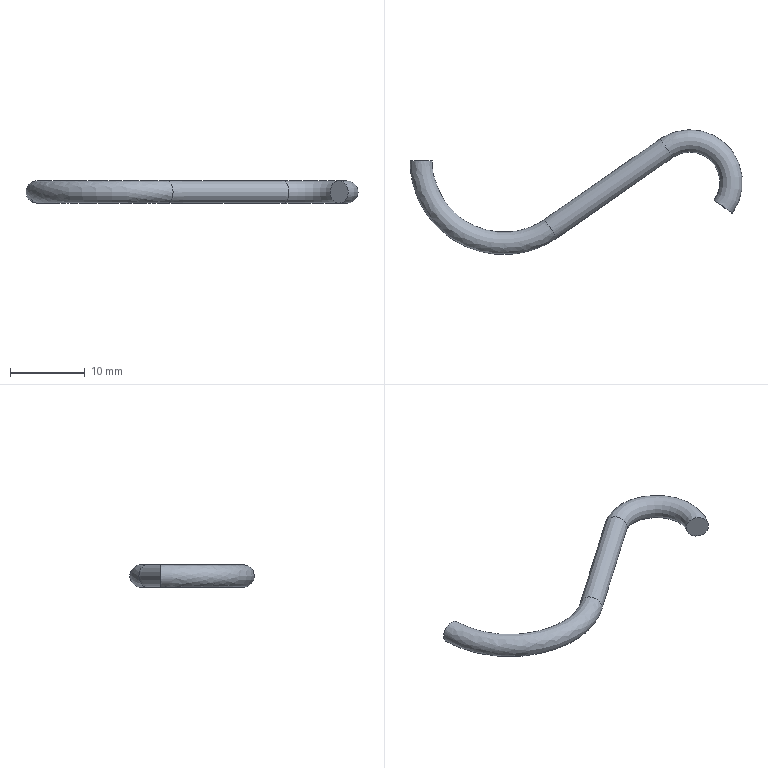Part | NX | features solid 2 | 1 solid | 5 faces | box 44.332 x 16.664 x 3 mm | volume 411.72 mm3 | spline 3 | plane 2
STEP:
#1=CARTESIAN_POINT('',(-1509.519,408.01,-17.5));
#2=VERTEX_POINT('',#1);
#3=CARTESIAN_POINT('',(-1510.727,408.9,-17.5));
#4=DIRECTION('',(-0.5934,-0.8049,0.));
#5=DIRECTION('',(0.8049,-0.5934,0.));
#6=AXIS2_PLACEMENT_3D('',#3,#4,#5);
#7=CIRCLE('',#6,1.5);
#8=EDGE_CURVE('',#2,#2,#7,.T.);
#9=ORIENTED_EDGE('',*,*,#8,.T.);
#10=EDGE_LOOP('',(#9));
#11=FACE_BOUND('',#10,.T.);
#12=CARTESIAN_POINT('',(-1510.727,408.9,-17.5));
#13=DIRECTION('',(0.5934,0.8049,0.));
#14=DIRECTION('',(-0.8049,0.5934,0.));
#15=AXIS2_PLACEMENT_3D('',#12,#13,#14);
#16=PLANE('',#15);
#17=ADVANCED_FACE('',(#11),#16,.F.);
#18=CARTESIAN_POINT('',(-1518.27,416.696,-16.));
#19=VERTEX_POINT('',#18);
#20=CARTESIAN_POINT('',(-1517.968,416.26,-16.));
#21=CARTESIAN_POINT('',(-1518.572,417.131,-16.));
#22=CARTESIAN_POINT('',(-1518.973,417.711,-16.265));
#23=CARTESIAN_POINT('',(-1519.124,417.929,-16.97));
#24=CARTESIAN_POINT('',(-1519.124,417.929,-18.03));
#25=CARTESIAN_POINT('',(-1518.973,417.711,-18.735));
#26=CARTESIAN_POINT('',(-1518.572,417.131,-19.));
#27=CARTESIAN_POINT('',(-1517.968,416.26,-19.));
#28=CARTESIAN_POINT('',(-1517.567,415.68,-18.735));
#29=CARTESIAN_POINT('',(-1517.416,415.462,-18.03));
#30=CARTESIAN_POINT('',(-1517.416,415.462,-16.97));
#31=CARTESIAN_POINT('',(-1517.567,415.68,-16.265));
#32=CARTESIAN_POINT('',(-1517.968,416.26,-16.));
#33=CARTESIAN_POINT('',(-1518.572,417.131,-16.));
#34=(BOUNDED_CURVE()B_SPLINE_CURVE(4,(#20,#21,#22,#23,#24,#25,#26,#27,#28,#29,#30,#31,#32,#33),.UNSPECIFIED.,.T.,.F.)B_SPLINE_CURVE_WITH_KNOTS((2,3,3,3,3,3,2),(-0.25,0.,0.25,0.5,0.75,1.,1.25),.UNSPECIFIED.)CURVE()GEOMETRIC_REPRESENTATION_ITEM()RATIONAL_B_SPLINE_CURVE((1.017,1.017,0.9585,1.017,1.017,0.9585,1.017,1.017,0.9585,1.017,1.017,0.9585,1.017,1.017))REPRESENTATION_ITEM(''));
#35=EDGE_CURVE('',#19,#19,#34,.F.);
#36=ORIENTED_EDGE('',*,*,#35,.T.);
#37=EDGE_LOOP('',(#36));
#38=FACE_BOUND('',#37,.T.);
#39=ORIENTED_EDGE('',*,*,#8,.F.);
#40=EDGE_LOOP('',(#39));
#41=FACE_BOUND('',#40,.T.);
#42=CARTESIAN_POINT('',(-1517.968,416.26,-16.));
#43=CARTESIAN_POINT('',(-1517.914,416.296,-16.));
#44=CARTESIAN_POINT('',(-1517.863,416.33,-16.));
#45=CARTESIAN_POINT('',(-1517.478,416.575,-16.));
#46=CARTESIAN_POINT('',(-1516.983,416.819,-16.));
#47=CARTESIAN_POINT('',(-1515.796,417.144,-16.));
#48=CARTESIAN_POINT('',(-1514.851,417.214,-16.));
#49=CARTESIAN_POINT('',(-1513.213,416.821,-16.));
#50=CARTESIAN_POINT('',(-1512.432,416.392,-16.));
#51=CARTESIAN_POINT('',(-1511.306,415.394,-16.));
#52=CARTESIAN_POINT('',(-1509.795,413.389,-16.));
#53=CARTESIAN_POINT('',(-1510.171,410.387,-16.));
#54=CARTESIAN_POINT('',(-1511.153,409.215,-16.));
#55=CARTESIAN_POINT('',(-1518.572,417.131,-16.));
#56=CARTESIAN_POINT('',(-1518.513,417.171,-16.));
#57=CARTESIAN_POINT('',(-1518.454,417.21,-16.));
#58=CARTESIAN_POINT('',(-1517.931,417.546,-16.));
#59=CARTESIAN_POINT('',(-1517.422,417.778,-16.));
#60=CARTESIAN_POINT('',(-1515.889,418.237,-16.));
#61=CARTESIAN_POINT('',(-1514.813,418.274,-16.));
#62=CARTESIAN_POINT('',(-1512.795,417.818,-16.));
#63=CARTESIAN_POINT('',(-1511.852,417.295,-16.));
#64=CARTESIAN_POINT('',(-1510.485,416.084,-16.));
#65=CARTESIAN_POINT('',(-1508.652,413.65,-16.));
#66=CARTESIAN_POINT('',(-1509.108,410.008,-16.));
#67=CARTESIAN_POINT('',(-1510.3,408.585,-16.));
#68=CARTESIAN_POINT('',(-1518.973,417.711,-16.265));
#69=CARTESIAN_POINT('',(-1518.912,417.752,-16.265));
#70=CARTESIAN_POINT('',(-1518.847,417.795,-16.265));
#71=CARTESIAN_POINT('',(-1518.232,418.191,-16.265));
#72=CARTESIAN_POINT('',(-1517.715,418.416,-16.265));
#73=CARTESIAN_POINT('',(-1515.951,418.963,-16.265));
#74=CARTESIAN_POINT('',(-1514.788,418.977,-16.265));
#75=CARTESIAN_POINT('',(-1512.516,418.481,-16.265));
#76=CARTESIAN_POINT('',(-1511.466,417.894,-16.265));
#77=CARTESIAN_POINT('',(-1509.939,416.542,-16.265));
#78=CARTESIAN_POINT('',(-1507.892,413.824,-16.265));
#79=CARTESIAN_POINT('',(-1508.402,409.757,-16.265));
#80=CARTESIAN_POINT('',(-1509.733,408.167,-16.265));
#81=CARTESIAN_POINT('',(-1519.124,417.929,-16.97));
#82=CARTESIAN_POINT('',(-1519.061,417.971,-16.97));
#83=CARTESIAN_POINT('',(-1518.994,418.016,-16.97));
#84=CARTESIAN_POINT('',(-1518.346,418.434,-16.97));
#85=CARTESIAN_POINT('',(-1517.824,418.655,-16.97));
#86=CARTESIAN_POINT('',(-1515.974,419.237,-16.97));
#87=CARTESIAN_POINT('',(-1514.779,419.242,-16.97));
#88=CARTESIAN_POINT('',(-1512.412,418.73,-16.97));
#89=CARTESIAN_POINT('',(-1511.321,418.12,-16.97));
#90=CARTESIAN_POINT('',(-1509.734,416.714,-16.97));
#91=CARTESIAN_POINT('',(-1507.606,413.89,-16.97));
#92=CARTESIAN_POINT('',(-1508.136,409.662,-16.97));
#93=CARTESIAN_POINT('',(-1509.519,408.01,-16.97));
#94=CARTESIAN_POINT('',(-1519.124,417.929,-18.03));
#95=CARTESIAN_POINT('',(-1519.061,417.971,-18.03));
#96=CARTESIAN_POINT('',(-1518.994,418.016,-18.03));
#97=CARTESIAN_POINT('',(-1518.346,418.434,-18.03));
#98=CARTESIAN_POINT('',(-1517.824,418.655,-18.03));
#99=CARTESIAN_POINT('',(-1515.974,419.237,-18.03));
#100=CARTESIAN_POINT('',(-1514.779,419.242,-18.03));
#101=CARTESIAN_POINT('',(-1512.412,418.73,-18.03));
#102=CARTESIAN_POINT('',(-1511.321,418.12,-18.03));
#103=CARTESIAN_POINT('',(-1509.734,416.714,-18.03));
#104=CARTESIAN_POINT('',(-1507.606,413.89,-18.03));
#105=CARTESIAN_POINT('',(-1508.136,409.662,-18.03));
#106=CARTESIAN_POINT('',(-1509.519,408.01,-18.03));
#107=CARTESIAN_POINT('',(-1518.973,417.711,-18.735));
#108=CARTESIAN_POINT('',(-1518.912,417.752,-18.735));
#109=CARTESIAN_POINT('',(-1518.847,417.795,-18.735));
#110=CARTESIAN_POINT('',(-1518.232,418.191,-18.735));
#111=CARTESIAN_POINT('',(-1517.715,418.416,-18.735));
#112=CARTESIAN_POINT('',(-1515.951,418.963,-18.735));
#113=CARTESIAN_POINT('',(-1514.788,418.977,-18.735));
#114=CARTESIAN_POINT('',(-1512.516,418.481,-18.735));
#115=CARTESIAN_POINT('',(-1511.466,417.894,-18.735));
#116=CARTESIAN_POINT('',(-1509.939,416.542,-18.735));
#117=CARTESIAN_POINT('',(-1507.892,413.824,-18.735));
#118=CARTESIAN_POINT('',(-1508.402,409.757,-18.735));
#119=CARTESIAN_POINT('',(-1509.733,408.167,-18.735));
#120=CARTESIAN_POINT('',(-1518.572,417.131,-19.));
#121=CARTESIAN_POINT('',(-1518.513,417.171,-19.));
#122=CARTESIAN_POINT('',(-1518.454,417.21,-19.));
#123=CARTESIAN_POINT('',(-1517.931,417.546,-19.));
#124=CARTESIAN_POINT('',(-1517.422,417.778,-19.));
#125=CARTESIAN_POINT('',(-1515.889,418.237,-19.));
#126=CARTESIAN_POINT('',(-1514.813,418.274,-19.));
#127=CARTESIAN_POINT('',(-1512.795,417.818,-19.));
#128=CARTESIAN_POINT('',(-1511.852,417.295,-19.));
#129=CARTESIAN_POINT('',(-1510.485,416.084,-19.));
#130=CARTESIAN_POINT('',(-1508.652,413.65,-19.));
#131=CARTESIAN_POINT('',(-1509.108,410.008,-19.));
#132=CARTESIAN_POINT('',(-1510.3,408.585,-19.));
#133=CARTESIAN_POINT('',(-1517.968,416.26,-19.));
#134=CARTESIAN_POINT('',(-1517.914,416.296,-19.));
#135=CARTESIAN_POINT('',(-1517.863,416.33,-19.));
#136=CARTESIAN_POINT('',(-1517.478,416.575,-19.));
#137=CARTESIAN_POINT('',(-1516.983,416.819,-19.));
#138=CARTESIAN_POINT('',(-1515.796,417.144,-19.));
#139=CARTESIAN_POINT('',(-1514.851,417.214,-19.));
#140=CARTESIAN_POINT('',(-1513.213,416.821,-19.));
#141=CARTESIAN_POINT('',(-1512.432,416.392,-19.));
#142=CARTESIAN_POINT('',(-1511.306,415.394,-19.));
#143=CARTESIAN_POINT('',(-1509.795,413.389,-19.));
#144=CARTESIAN_POINT('',(-1510.171,410.387,-19.));
#145=CARTESIAN_POINT('',(-1511.153,409.215,-19.));
#146=CARTESIAN_POINT('',(-1517.567,415.68,-18.735));
#147=CARTESIAN_POINT('',(-1517.516,415.715,-18.735));
#148=CARTESIAN_POINT('',(-1517.471,415.745,-18.735));
#149=CARTESIAN_POINT('',(-1517.176,415.93,-18.735));
#150=CARTESIAN_POINT('',(-1516.691,416.182,-18.735));
#151=CARTESIAN_POINT('',(-1515.734,416.418,-18.735));
#152=CARTESIAN_POINT('',(-1514.875,416.511,-18.735));
#153=CARTESIAN_POINT('',(-1513.492,416.159,-18.735));
#154=CARTESIAN_POINT('',(-1512.818,415.793,-18.735));
#155=CARTESIAN_POINT('',(-1511.851,414.936,-18.735));
#156=CARTESIAN_POINT('',(-1510.555,413.215,-18.735));
#157=CARTESIAN_POINT('',(-1510.878,410.639,-18.735));
#158=CARTESIAN_POINT('',(-1511.721,409.633,-18.735));
#159=CARTESIAN_POINT('',(-1517.416,415.462,-18.03));
#160=CARTESIAN_POINT('',(-1517.366,415.496,-18.03));
#161=CARTESIAN_POINT('',(-1517.323,415.525,-18.03));
#162=CARTESIAN_POINT('',(-1517.063,415.688,-18.03));
#163=CARTESIAN_POINT('',(-1516.581,415.942,-18.03));
#164=CARTESIAN_POINT('',(-1515.71,416.145,-18.03));
#165=CARTESIAN_POINT('',(-1514.885,416.246,-18.03));
#166=CARTESIAN_POINT('',(-1513.596,415.909,-18.03));
#167=CARTESIAN_POINT('',(-1512.963,415.568,-18.03));
#168=CARTESIAN_POINT('',(-1512.057,414.764,-18.03));
#169=CARTESIAN_POINT('',(-1510.841,413.15,-18.03));
#170=CARTESIAN_POINT('',(-1511.144,410.734,-18.03));
#171=CARTESIAN_POINT('',(-1511.934,409.79,-18.03));
#172=CARTESIAN_POINT('',(-1517.416,415.462,-16.97));
#173=CARTESIAN_POINT('',(-1517.366,415.496,-16.97));
#174=CARTESIAN_POINT('',(-1517.323,415.525,-16.97));
#175=CARTESIAN_POINT('',(-1517.063,415.688,-16.97));
#176=CARTESIAN_POINT('',(-1516.581,415.942,-16.97));
#177=CARTESIAN_POINT('',(-1515.71,416.145,-16.97));
#178=CARTESIAN_POINT('',(-1514.885,416.246,-16.97));
#179=CARTESIAN_POINT('',(-1513.596,415.909,-16.97));
#180=CARTESIAN_POINT('',(-1512.963,415.568,-16.97));
#181=CARTESIAN_POINT('',(-1512.057,414.764,-16.97));
#182=CARTESIAN_POINT('',(-1510.841,413.15,-16.97));
#183=CARTESIAN_POINT('',(-1511.144,410.734,-16.97));
#184=CARTESIAN_POINT('',(-1511.934,409.79,-16.97));
#185=CARTESIAN_POINT('',(-1517.567,415.68,-16.265));
#186=CARTESIAN_POINT('',(-1517.516,415.715,-16.265));
#187=CARTESIAN_POINT('',(-1517.471,415.745,-16.265));
#188=CARTESIAN_POINT('',(-1517.176,415.93,-16.265));
#189=CARTESIAN_POINT('',(-1516.691,416.182,-16.265));
#190=CARTESIAN_POINT('',(-1515.734,416.418,-16.265));
#191=CARTESIAN_POINT('',(-1514.875,416.511,-16.265));
#192=CARTESIAN_POINT('',(-1513.492,416.159,-16.265));
#193=CARTESIAN_POINT('',(-1512.818,415.793,-16.265));
#194=CARTESIAN_POINT('',(-1511.851,414.936,-16.265));
#195=CARTESIAN_POINT('',(-1510.555,413.215,-16.265));
#196=CARTESIAN_POINT('',(-1510.878,410.639,-16.265));
#197=CARTESIAN_POINT('',(-1511.721,409.633,-16.265));
#198=CARTESIAN_POINT('',(-1517.968,416.26,-16.));
#199=CARTESIAN_POINT('',(-1517.914,416.296,-16.));
#200=CARTESIAN_POINT('',(-1517.863,416.33,-16.));
#201=CARTESIAN_POINT('',(-1517.478,416.575,-16.));
#202=CARTESIAN_POINT('',(-1516.983,416.819,-16.));
#203=CARTESIAN_POINT('',(-1515.796,417.144,-16.));
#204=CARTESIAN_POINT('',(-1514.851,417.214,-16.));
#205=CARTESIAN_POINT('',(-1513.213,416.821,-16.));
#206=CARTESIAN_POINT('',(-1512.432,416.392,-16.));
#207=CARTESIAN_POINT('',(-1511.306,415.394,-16.));
#208=CARTESIAN_POINT('',(-1509.795,413.389,-16.));
#209=CARTESIAN_POINT('',(-1510.171,410.387,-16.));
#210=CARTESIAN_POINT('',(-1511.153,409.215,-16.));
#211=CARTESIAN_POINT('',(-1518.572,417.131,-16.));
#212=CARTESIAN_POINT('',(-1518.513,417.171,-16.));
#213=CARTESIAN_POINT('',(-1518.454,417.21,-16.));
#214=CARTESIAN_POINT('',(-1517.931,417.546,-16.));
#215=CARTESIAN_POINT('',(-1517.422,417.778,-16.));
#216=CARTESIAN_POINT('',(-1515.889,418.237,-16.));
#217=CARTESIAN_POINT('',(-1514.813,418.274,-16.));
#218=CARTESIAN_POINT('',(-1512.795,417.818,-16.));
#219=CARTESIAN_POINT('',(-1511.852,417.295,-16.));
#220=CARTESIAN_POINT('',(-1510.485,416.084,-16.));
#221=CARTESIAN_POINT('',(-1508.652,413.65,-16.));
#222=CARTESIAN_POINT('',(-1509.108,410.008,-16.));
#223=CARTESIAN_POINT('',(-1510.3,408.585,-16.));
#224=(BOUNDED_SURFACE()B_SPLINE_SURFACE(4,3,((#42,#43,#44,#45,#46,#47,#48,#49,#50,#51,#52,#53,#54),(#55,#56,#57,#58,#59,#60,#61,#62,#63,#64,#65,#66,#67),(#68,#69,#70,#71,#72,#73,#74,#75,#76,#77,#78,#79,#80),(#81,#82,#83,#84,#85,#86,#87,#88,#89,#90,#91,#92,#93),(#94,#95,#96,#97,#98,#99,#100,#101,#102,#103,#104,#105,#106),(#107,#108,#109,#110,#111,#112,#113,#114,#115,#116,#117,#118,#119),(#120,#121,#122,#123,#124,#125,#126,#127,#128,#129,#130,#131,#132),(#133,#134,#135,#136,#137,#138,#139,#140,#141,#142,#143,#144,#145),(#146,#147,#148,#149,#150,#151,#152,#153,#154,#155,#156,#157,#158),(#159,#160,#161,#162,#163,#164,#165,#166,#167,#168,#169,#170,#171),(#172,#173,#174,#175,#176,#177,#178,#179,#180,#181,#182,#183,#184),(#185,#186,#187,#188,#189,#190,#191,#192,#193,#194,#195,#196,#197),(#198,#199,#200,#201,#202,#203,#204,#205,#206,#207,#208,#209,#210),(#211,#212,#213,#214,#215,#216,#217,#218,#219,#220,#221,#222,#223)),.UNSPECIFIED.,.T.,.F.,.F.)B_SPLINE_SURFACE_WITH_KNOTS((2,3,3,3,3,3,2),(4,2,2,2,2,1,4),(-0.25,0.,0.25,0.5,0.75,1.,1.25),(0.,0.01356,0.1166,0.2933,0.47,0.6466,1.),.UNSPECIFIED.)GEOMETRIC_REPRESENTATION_ITEM()RATIONAL_B_SPLINE_SURFACE(((1.017,1.017,1.017,1.017,1.017,1.017,1.017,1.017,1.017,1.017,1.017,1.017,1.017),(1.017,1.017,1.017,1.017,1.017,1.017,1.017,1.017,1.017,1.017,1.017,1.017,1.017),(0.9585,0.9585,0.9585,0.9585,0.9585,0.9585,0.9585,0.9585,0.9585,0.9585,0.9585,0.9585,0.9585),(1.017,1.017,1.017,1.017,1.017,1.017,1.017,1.017,1.017,1.017,1.017,1.017,1.017),(1.017,1.017,1.017,1.017,1.017,1.017,1.017,1.017,1.017,1.017,1.017,1.017,1.017),(0.9585,0.9585,0.9585,0.9585,0.9585,0.9585,0.9585,0.9585,0.9585,0.9585,0.9585,0.9585,0.9585),(1.017,1.017,1.017,1.017,1.017,1.017,1.017,1.017,1.017,1.017,1.017,1.017,1.017),(1.017,1.017,1.017,1.017,1.017,1.017,1.017,1.017,1.017,1.017,1.017,1.017,1.017),(0.9585,0.9585,0.9585,0.9585,0.9585,0.9585,0.9585,0.9585,0.9585,0.9585,0.9585,0.9585,0.9585),(1.017,1.017,1.017,1.017,1.017,1.017,1.017,1.017,1.017,1.017,1.017,1.017,1.017),(1.017,1.017,1.017,1.017,1.017,1.017,1.017,1.017,1.017,1.017,1.017,1.017,1.017),(0.9585,0.9585,0.9585,0.9585,0.9585,0.9585,0.9585,0.9585,0.9585,0.9585,0.9585,0.9585,0.9585),(1.017,1.017,1.017,1.017,1.017,1.017,1.017,1.017,1.017,1.017,1.017,1.017,1.017),(1.017,1.017,1.017,1.017,1.017,1.017,1.017,1.017,1.017,1.017,1.017,1.017,1.017)))REPRESENTATION_ITEM('')SURFACE());
#225=ADVANCED_FACE('',(#38,#41),#224,.F.);
#226=CARTESIAN_POINT('',(-1533.724,405.97,-16.));
#227=VERTEX_POINT('',#226);
#228=CARTESIAN_POINT('',(-1533.427,405.531,-16.));
#229=CARTESIAN_POINT('',(-1534.021,406.409,-16.));
#230=CARTESIAN_POINT('',(-1534.416,406.992,-16.265));
#231=CARTESIAN_POINT('',(-1534.564,407.212,-16.97));
#232=CARTESIAN_POINT('',(-1534.564,407.212,-18.03));
#233=CARTESIAN_POINT('',(-1534.416,406.992,-18.735));
#234=CARTESIAN_POINT('',(-1534.021,406.409,-19.));
#235=CARTESIAN_POINT('',(-1533.427,405.531,-19.));
#236=CARTESIAN_POINT('',(-1533.032,404.947,-18.735));
#237=CARTESIAN_POINT('',(-1532.883,404.728,-18.03));
#238=CARTESIAN_POINT('',(-1532.883,404.728,-16.97));
#239=CARTESIAN_POINT('',(-1533.032,404.947,-16.265));
#240=CARTESIAN_POINT('',(-1533.427,405.531,-16.));
#241=CARTESIAN_POINT('',(-1534.021,406.409,-16.));
#242=(BOUNDED_CURVE()B_SPLINE_CURVE(4,(#228,#229,#230,#231,#232,#233,#234,#235,#236,#237,#238,#239,#240,#241),.UNSPECIFIED.,.T.,.F.)B_SPLINE_CURVE_WITH_KNOTS((2,3,3,3,3,3,2),(-0.25,0.,0.25,0.5,0.75,1.,1.25),.UNSPECIFIED.)CURVE()GEOMETRIC_REPRESENTATION_ITEM()RATIONAL_B_SPLINE_CURVE((1.017,1.017,0.9585,1.017,1.017,0.9585,1.017,1.017,0.9585,1.017,1.017,0.9585,1.017,1.017))REPRESENTATION_ITEM(''));
#243=EDGE_CURVE('',#227,#227,#242,.F.);
#244=ORIENTED_EDGE('',*,*,#243,.T.);
#245=EDGE_LOOP('',(#244));
#246=FACE_BOUND('',#245,.T.);
#247=ORIENTED_EDGE('',*,*,#35,.F.);
#248=EDGE_LOOP('',(#247));
#249=FACE_BOUND('',#248,.T.);
#250=CARTESIAN_POINT('',(-1533.427,405.531,-16.));
#251=CARTESIAN_POINT('',(-1532.754,405.985,-16.));
#252=CARTESIAN_POINT('',(-1532.099,406.453,-16.));
#253=CARTESIAN_POINT('',(-1530.183,407.774,-16.));
#254=CARTESIAN_POINT('',(-1528.943,408.643,-16.));
#255=CARTESIAN_POINT('',(-1526.699,410.197,-16.));
#256=CARTESIAN_POINT('',(-1525.703,410.889,-16.));
#257=CARTESIAN_POINT('',(-1523.213,412.618,-16.));
#258=CARTESIAN_POINT('',(-1521.717,413.657,-16.));
#259=CARTESIAN_POINT('',(-1519.603,415.124,-16.));
#260=CARTESIAN_POINT('',(-1518.976,415.56,-16.));
#261=CARTESIAN_POINT('',(-1518.228,416.078,-16.));
#262=CARTESIAN_POINT('',(-1518.09,416.177,-16.));
#263=CARTESIAN_POINT('',(-1517.968,416.26,-16.));
#264=CARTESIAN_POINT('',(-1534.021,406.409,-16.));
#265=CARTESIAN_POINT('',(-1533.386,406.838,-16.));
#266=CARTESIAN_POINT('',(-1532.691,407.333,-16.));
#267=CARTESIAN_POINT('',(-1530.803,408.635,-16.));
#268=CARTESIAN_POINT('',(-1529.539,409.52,-16.));
#269=CARTESIAN_POINT('',(-1527.307,411.066,-16.));
#270=CARTESIAN_POINT('',(-1526.308,411.761,-16.));
#271=CARTESIAN_POINT('',(-1523.817,413.49,-16.));
#272=CARTESIAN_POINT('',(-1522.323,414.527,-16.));
#273=CARTESIAN_POINT('',(-1520.205,415.997,-16.));
#274=CARTESIAN_POINT('',(-1519.584,416.43,-16.));
#275=CARTESIAN_POINT('',(-1518.83,416.952,-16.));
#276=CARTESIAN_POINT('',(-1518.703,417.042,-16.));
#277=CARTESIAN_POINT('',(-1518.572,417.131,-16.));
#278=CARTESIAN_POINT('',(-1534.416,406.992,-16.265));
#279=CARTESIAN_POINT('',(-1533.805,407.405,-16.265));
#280=CARTESIAN_POINT('',(-1533.084,407.918,-16.265));
#281=CARTESIAN_POINT('',(-1531.215,409.207,-16.265));
#282=CARTESIAN_POINT('',(-1529.935,410.102,-16.265));
#283=CARTESIAN_POINT('',(-1527.711,411.643,-16.265));
#284=CARTESIAN_POINT('',(-1526.709,412.34,-16.265));
#285=CARTESIAN_POINT('',(-1524.219,414.069,-16.265));
#286=CARTESIAN_POINT('',(-1522.726,415.105,-16.265));
#287=CARTESIAN_POINT('',(-1520.605,416.577,-16.265));
#288=CARTESIAN_POINT('',(-1519.988,417.007,-16.265));
#289=CARTESIAN_POINT('',(-1519.23,417.532,-16.265));
#290=CARTESIAN_POINT('',(-1519.111,417.617,-16.265));
#291=CARTESIAN_POINT('',(-1518.973,417.711,-16.265));
#292=CARTESIAN_POINT('',(-1534.564,407.212,-16.97));
#293=CARTESIAN_POINT('',(-1533.963,407.619,-16.97));
#294=CARTESIAN_POINT('',(-1533.232,408.138,-16.97));
#295=CARTESIAN_POINT('',(-1531.37,409.422,-16.97));
#296=CARTESIAN_POINT('',(-1530.084,410.322,-16.97));
#297=CARTESIAN_POINT('',(-1527.863,411.86,-16.97));
#298=CARTESIAN_POINT('',(-1526.861,412.557,-16.97));
#299=CARTESIAN_POINT('',(-1524.37,414.286,-16.97));
#300=CARTESIAN_POINT('',(-1522.878,415.323,-16.97));
#301=CARTESIAN_POINT('',(-1520.756,416.795,-16.97));
#302=CARTESIAN_POINT('',(-1520.14,417.224,-16.97));
#303=CARTESIAN_POINT('',(-1519.381,417.75,-16.97));
#304=CARTESIAN_POINT('',(-1519.265,417.833,-16.97));
#305=CARTESIAN_POINT('',(-1519.124,417.929,-16.97));
#306=CARTESIAN_POINT('',(-1534.564,407.212,-18.03));
#307=CARTESIAN_POINT('',(-1533.963,407.619,-18.03));
#308=CARTESIAN_POINT('',(-1533.232,408.138,-18.03));
#309=CARTESIAN_POINT('',(-1531.37,409.422,-18.03));
#310=CARTESIAN_POINT('',(-1530.084,410.322,-18.03));
#311=CARTESIAN_POINT('',(-1527.863,411.86,-18.03));
#312=CARTESIAN_POINT('',(-1526.861,412.557,-18.03));
#313=CARTESIAN_POINT('',(-1524.37,414.286,-18.03));
#314=CARTESIAN_POINT('',(-1522.878,415.323,-18.03));
#315=CARTESIAN_POINT('',(-1520.756,416.795,-18.03));
#316=CARTESIAN_POINT('',(-1520.14,417.224,-18.03));
#317=CARTESIAN_POINT('',(-1519.381,417.75,-18.03));
#318=CARTESIAN_POINT('',(-1519.265,417.833,-18.03));
#319=CARTESIAN_POINT('',(-1519.124,417.929,-18.03));
#320=CARTESIAN_POINT('',(-1534.416,406.992,-18.735));
#321=CARTESIAN_POINT('',(-1533.805,407.405,-18.735));
#322=CARTESIAN_POINT('',(-1533.084,407.918,-18.735));
#323=CARTESIAN_POINT('',(-1531.215,409.207,-18.735));
#324=CARTESIAN_POINT('',(-1529.935,410.102,-18.735));
#325=CARTESIAN_POINT('',(-1527.711,411.643,-18.735));
#326=CARTESIAN_POINT('',(-1526.709,412.34,-18.735));
#327=CARTESIAN_POINT('',(-1524.219,414.069,-18.735));
#328=CARTESIAN_POINT('',(-1522.726,415.105,-18.735));
#329=CARTESIAN_POINT('',(-1520.605,416.577,-18.735));
#330=CARTESIAN_POINT('',(-1519.988,417.007,-18.735));
#331=CARTESIAN_POINT('',(-1519.23,417.532,-18.735));
#332=CARTESIAN_POINT('',(-1519.111,417.617,-18.735));
#333=CARTESIAN_POINT('',(-1518.973,417.711,-18.735));
#334=CARTESIAN_POINT('',(-1534.021,406.409,-19.));
#335=CARTESIAN_POINT('',(-1533.386,406.838,-19.));
#336=CARTESIAN_POINT('',(-1532.691,407.333,-19.));
#337=CARTESIAN_POINT('',(-1530.803,408.635,-19.));
#338=CARTESIAN_POINT('',(-1529.539,409.52,-19.));
#339=CARTESIAN_POINT('',(-1527.307,411.066,-19.));
#340=CARTESIAN_POINT('',(-1526.308,411.761,-19.));
#341=CARTESIAN_POINT('',(-1523.817,413.49,-19.));
#342=CARTESIAN_POINT('',(-1522.323,414.527,-19.));
#343=CARTESIAN_POINT('',(-1520.205,415.997,-19.));
#344=CARTESIAN_POINT('',(-1519.584,416.43,-19.));
#345=CARTESIAN_POINT('',(-1518.83,416.952,-19.));
#346=CARTESIAN_POINT('',(-1518.703,417.042,-19.));
#347=CARTESIAN_POINT('',(-1518.572,417.131,-19.));
#348=CARTESIAN_POINT('',(-1533.427,405.531,-19.));
#349=CARTESIAN_POINT('',(-1532.754,405.985,-19.));
#350=CARTESIAN_POINT('',(-1532.099,406.453,-19.));
#351=CARTESIAN_POINT('',(-1530.183,407.774,-19.));
#352=CARTESIAN_POINT('',(-1528.943,408.643,-19.));
#353=CARTESIAN_POINT('',(-1526.699,410.197,-19.));
#354=CARTESIAN_POINT('',(-1525.703,410.889,-19.));
#355=CARTESIAN_POINT('',(-1523.213,412.618,-19.));
#356=CARTESIAN_POINT('',(-1521.717,413.657,-19.));
#357=CARTESIAN_POINT('',(-1519.603,415.124,-19.));
#358=CARTESIAN_POINT('',(-1518.976,415.56,-19.));
#359=CARTESIAN_POINT('',(-1518.228,416.078,-19.));
#360=CARTESIAN_POINT('',(-1518.09,416.177,-19.));
#361=CARTESIAN_POINT('',(-1517.968,416.26,-19.));
#362=CARTESIAN_POINT('',(-1533.032,404.947,-18.735));
#363=CARTESIAN_POINT('',(-1532.334,405.418,-18.735));
#364=CARTESIAN_POINT('',(-1531.706,405.869,-18.735));
#365=CARTESIAN_POINT('',(-1529.771,407.202,-18.735));
#366=CARTESIAN_POINT('',(-1528.547,408.06,-18.735));
#367=CARTESIAN_POINT('',(-1526.295,409.62,-18.735));
#368=CARTESIAN_POINT('',(-1525.301,410.311,-18.735));
#369=CARTESIAN_POINT('',(-1522.811,412.039,-18.735));
#370=CARTESIAN_POINT('',(-1521.314,413.079,-18.735));
#371=CARTESIAN_POINT('',(-1519.202,414.545,-18.735));
#372=CARTESIAN_POINT('',(-1518.572,414.983,-18.735));
#373=CARTESIAN_POINT('',(-1517.828,415.499,-18.735));
#374=CARTESIAN_POINT('',(-1517.682,415.602,-18.735));
#375=CARTESIAN_POINT('',(-1517.567,415.68,-18.735));
#376=CARTESIAN_POINT('',(-1532.883,404.728,-18.03));
#377=CARTESIAN_POINT('',(-1532.177,405.204,-18.03));
#378=CARTESIAN_POINT('',(-1531.558,405.649,-18.03));
#379=CARTESIAN_POINT('',(-1529.616,406.986,-18.03));
#380=CARTESIAN_POINT('',(-1528.398,407.841,-18.03));
#381=CARTESIAN_POINT('',(-1526.143,409.402,-18.03));
#382=CARTESIAN_POINT('',(-1525.15,410.093,-18.03));
#383=CARTESIAN_POINT('',(-1522.66,411.821,-18.03));
#384=CARTESIAN_POINT('',(-1521.162,412.862,-18.03));
#385=CARTESIAN_POINT('',(-1519.052,414.326,-18.03));
#386=CARTESIAN_POINT('',(-1518.42,414.766,-18.03));
#387=CARTESIAN_POINT('',(-1517.678,415.28,-18.03));
#388=CARTESIAN_POINT('',(-1517.528,415.386,-18.03));
#389=CARTESIAN_POINT('',(-1517.416,415.462,-18.03));
#390=CARTESIAN_POINT('',(-1532.883,404.728,-16.97));
#391=CARTESIAN_POINT('',(-1532.177,405.204,-16.97));
#392=CARTESIAN_POINT('',(-1531.558,405.649,-16.97));
#393=CARTESIAN_POINT('',(-1529.616,406.986,-16.97));
#394=CARTESIAN_POINT('',(-1528.398,407.841,-16.97));
#395=CARTESIAN_POINT('',(-1526.143,409.402,-16.97));
#396=CARTESIAN_POINT('',(-1525.15,410.093,-16.97));
#397=CARTESIAN_POINT('',(-1522.66,411.821,-16.97));
#398=CARTESIAN_POINT('',(-1521.162,412.862,-16.97));
#399=CARTESIAN_POINT('',(-1519.052,414.326,-16.97));
#400=CARTESIAN_POINT('',(-1518.42,414.766,-16.97));
#401=CARTESIAN_POINT('',(-1517.678,415.28,-16.97));
#402=CARTESIAN_POINT('',(-1517.528,415.386,-16.97));
#403=CARTESIAN_POINT('',(-1517.416,415.462,-16.97));
#404=CARTESIAN_POINT('',(-1533.032,404.947,-16.265));
#405=CARTESIAN_POINT('',(-1532.334,405.418,-16.265));
#406=CARTESIAN_POINT('',(-1531.706,405.869,-16.265));
#407=CARTESIAN_POINT('',(-1529.771,407.202,-16.265));
#408=CARTESIAN_POINT('',(-1528.547,408.06,-16.265));
#409=CARTESIAN_POINT('',(-1526.295,409.62,-16.265));
#410=CARTESIAN_POINT('',(-1525.301,410.311,-16.265));
#411=CARTESIAN_POINT('',(-1522.811,412.039,-16.265));
#412=CARTESIAN_POINT('',(-1521.314,413.079,-16.265));
#413=CARTESIAN_POINT('',(-1519.202,414.545,-16.265));
#414=CARTESIAN_POINT('',(-1518.572,414.983,-16.265));
#415=CARTESIAN_POINT('',(-1517.828,415.499,-16.265));
#416=CARTESIAN_POINT('',(-1517.682,415.602,-16.265));
#417=CARTESIAN_POINT('',(-1517.567,415.68,-16.265));
#418=CARTESIAN_POINT('',(-1533.427,405.531,-16.));
#419=CARTESIAN_POINT('',(-1532.754,405.985,-16.));
#420=CARTESIAN_POINT('',(-1532.099,406.453,-16.));
#421=CARTESIAN_POINT('',(-1530.183,407.774,-16.));
#422=CARTESIAN_POINT('',(-1528.943,408.643,-16.));
#423=CARTESIAN_POINT('',(-1526.699,410.197,-16.));
#424=CARTESIAN_POINT('',(-1525.703,410.889,-16.));
#425=CARTESIAN_POINT('',(-1523.213,412.618,-16.));
#426=CARTESIAN_POINT('',(-1521.717,413.657,-16.));
#427=CARTESIAN_POINT('',(-1519.603,415.124,-16.));
#428=CARTESIAN_POINT('',(-1518.976,415.56,-16.));
#429=CARTESIAN_POINT('',(-1518.228,416.078,-16.));
#430=CARTESIAN_POINT('',(-1518.09,416.177,-16.));
#431=CARTESIAN_POINT('',(-1517.968,416.26,-16.));
#432=CARTESIAN_POINT('',(-1534.021,406.409,-16.));
#433=CARTESIAN_POINT('',(-1533.386,406.838,-16.));
#434=CARTESIAN_POINT('',(-1532.691,407.333,-16.));
#435=CARTESIAN_POINT('',(-1530.803,408.635,-16.));
#436=CARTESIAN_POINT('',(-1529.539,409.52,-16.));
#437=CARTESIAN_POINT('',(-1527.307,411.066,-16.));
#438=CARTESIAN_POINT('',(-1526.308,411.761,-16.));
#439=CARTESIAN_POINT('',(-1523.817,413.49,-16.));
#440=CARTESIAN_POINT('',(-1522.323,414.527,-16.));
#441=CARTESIAN_POINT('',(-1520.205,415.997,-16.));
#442=CARTESIAN_POINT('',(-1519.584,416.43,-16.));
#443=CARTESIAN_POINT('',(-1518.83,416.952,-16.));
#444=CARTESIAN_POINT('',(-1518.703,417.042,-16.));
#445=CARTESIAN_POINT('',(-1518.572,417.131,-16.));
#446=(BOUNDED_SURFACE()B_SPLINE_SURFACE(4,3,((#250,#251,#252,#253,#254,#255,#256,#257,#258,#259,#260,#261,#262,#263),(#264,#265,#266,#267,#268,#269,#270,#271,#272,#273,#274,#275,#276,#277),(#278,#279,#280,#281,#282,#283,#284,#285,#286,#287,#288,#289,#290,#291),(#292,#293,#294,#295,#296,#297,#298,#299,#300,#301,#302,#303,#304,#305),(#306,#307,#308,#309,#310,#311,#312,#313,#314,#315,#316,#317,#318,#319),(#320,#321,#322,#323,#324,#325,#326,#327,#328,#329,#330,#331,#332,#333),(#334,#335,#336,#337,#338,#339,#340,#341,#342,#343,#344,#345,#346,#347),(#348,#349,#350,#351,#352,#353,#354,#355,#356,#357,#358,#359,#360,#361),(#362,#363,#364,#365,#366,#367,#368,#369,#370,#371,#372,#373,#374,#375),(#376,#377,#378,#379,#380,#381,#382,#383,#384,#385,#386,#387,#388,#389),(#390,#391,#392,#393,#394,#395,#396,#397,#398,#399,#400,#401,#402,#403),(#404,#405,#406,#407,#408,#409,#410,#411,#412,#413,#414,#415,#416,#417),(#418,#419,#420,#421,#422,#423,#424,#425,#426,#427,#428,#429,#430,#431),(#432,#433,#434,#435,#436,#437,#438,#439,#440,#441,#442,#443,#444,#445)),.UNSPECIFIED.,.T.,.F.,.F.)B_SPLINE_SURFACE_WITH_KNOTS((2,3,3,3,3,3,2),(4,2,2,2,2,2,4),(-0.25,0.,0.25,0.5,0.75,1.,1.25),(0.,0.1289,0.3706,0.564,0.854,0.9749,1.),.UNSPECIFIED.)GEOMETRIC_REPRESENTATION_ITEM()RATIONAL_B_SPLINE_SURFACE(((1.017,1.017,1.017,1.017,1.017,1.017,1.017,1.017,1.017,1.017,1.017,1.017,1.017,1.017),(1.017,1.017,1.017,1.017,1.017,1.017,1.017,1.017,1.017,1.017,1.017,1.017,1.017,1.017),(0.9585,0.9585,0.9585,0.9585,0.9585,0.9585,0.9585,0.9585,0.9585,0.9585,0.9585,0.9585,0.9585,0.9585),(1.017,1.017,1.017,1.017,1.017,1.017,1.017,1.017,1.017,1.017,1.017,1.017,1.017,1.017),(1.017,1.017,1.017,1.017,1.017,1.017,1.017,1.017,1.017,1.017,1.017,1.017,1.017,1.017),(0.9585,0.9585,0.9585,0.9585,0.9585,0.9585,0.9585,0.9585,0.9585,0.9585,0.9585,0.9585,0.9585,0.9585),(1.017,1.017,1.017,1.017,1.017,1.017,1.017,1.017,1.017,1.017,1.017,1.017,1.017,1.017),(1.017,1.017,1.017,1.017,1.017,1.017,1.017,1.017,1.017,1.017,1.017,1.017,1.017,1.017),(0.9585,0.9585,0.9585,0.9585,0.9585,0.9585,0.9585,0.9585,0.9585,0.9585,0.9585,0.9585,0.9585,0.9585),(1.017,1.017,1.017,1.017,1.017,1.017,1.017,1.017,1.017,1.017,1.017,1.017,1.017,1.017),(1.017,1.017,1.017,1.017,1.017,1.017,1.017,1.017,1.017,1.017,1.017,1.017,1.017,1.017),(0.9585,0.9585,0.9585,0.9585,0.9585,0.9585,0.9585,0.9585,0.9585,0.9585,0.9585,0.9585,0.9585,0.9585),(1.017,1.017,1.017,1.017,1.017,1.017,1.017,1.017,1.017,1.017,1.017,1.017,1.017,1.017),(1.017,1.017,1.017,1.017,1.017,1.017,1.017,1.017,1.017,1.017,1.017,1.017,1.017,1.017)))REPRESENTATION_ITEM('')SURFACE());
#447=ADVANCED_FACE('',(#246,#249),#446,.F.);
#448=CARTESIAN_POINT('',(-1552.5,415.,-17.5));
#449=VERTEX_POINT('',#448);
#450=CARTESIAN_POINT('',(-1551.,415.,-17.5));
#451=DIRECTION('',(0.,1.,0.));
#452=DIRECTION('',(-1.,0.,0.));
#453=AXIS2_PLACEMENT_3D('',#450,#451,#452);
#454=CIRCLE('',#453,1.5);
#455=EDGE_CURVE('',#449,#449,#454,.T.);
#456=ORIENTED_EDGE('',*,*,#455,.T.);
#457=EDGE_LOOP('',(#456));
#458=FACE_BOUND('',#457,.T.);
#459=CARTESIAN_POINT('',(-1551.,415.,-17.5));
#460=DIRECTION('',(0.,-1.,0.));
#461=DIRECTION('',(1.,0.,0.));
#462=AXIS2_PLACEMENT_3D('',#459,#460,#461);
#463=PLANE('',#462);
#464=ADVANCED_FACE('',(#458),#463,.F.);
#465=ORIENTED_EDGE('',*,*,#455,.F.);
#466=EDGE_LOOP('',(#465));
#467=FACE_BOUND('',#466,.T.);
#468=ORIENTED_EDGE('',*,*,#243,.F.);
#469=EDGE_LOOP('',(#468));
#470=FACE_BOUND('',#469,.T.);
#471=CARTESIAN_POINT('',(-1551.53,415.,-16.));
#472=CARTESIAN_POINT('',(-1551.546,413.187,-16.));
#473=CARTESIAN_POINT('',(-1551.071,411.245,-16.));
#474=CARTESIAN_POINT('',(-1549.226,407.799,-16.));
#475=CARTESIAN_POINT('',(-1547.821,406.325,-16.));
#476=CARTESIAN_POINT('',(-1544.216,403.994,-16.));
#477=CARTESIAN_POINT('',(-1541.701,403.292,-16.));
#478=CARTESIAN_POINT('',(-1537.066,403.672,-16.));
#479=CARTESIAN_POINT('',(-1535.204,404.349,-16.));
#480=CARTESIAN_POINT('',(-1533.595,405.417,-16.));
#481=CARTESIAN_POINT('',(-1533.511,405.474,-16.));
#482=CARTESIAN_POINT('',(-1533.427,405.531,-16.));
#483=CARTESIAN_POINT('',(-1550.47,415.,-16.));
#484=CARTESIAN_POINT('',(-1550.484,413.354,-16.));
#485=CARTESIAN_POINT('',(-1550.053,411.591,-16.));
#486=CARTESIAN_POINT('',(-1548.377,408.462,-16.));
#487=CARTESIAN_POINT('',(-1547.102,407.123,-16.));
#488=CARTESIAN_POINT('',(-1543.829,405.006,-16.));
#489=CARTESIAN_POINT('',(-1541.545,404.369,-16.));
#490=CARTESIAN_POINT('',(-1537.335,404.714,-16.));
#491=CARTESIAN_POINT('',(-1535.649,405.326,-16.));
#492=CARTESIAN_POINT('',(-1534.179,406.303,-16.));
#493=CARTESIAN_POINT('',(-1534.1,406.355,-16.));
#494=CARTESIAN_POINT('',(-1534.021,406.409,-16.));
#495=CARTESIAN_POINT('',(-1549.765,415.,-16.265));
#496=CARTESIAN_POINT('',(-1549.778,413.464,-16.265));
#497=CARTESIAN_POINT('',(-1549.376,411.82,-16.265));
#498=CARTESIAN_POINT('',(-1547.813,408.902,-16.265));
#499=CARTESIAN_POINT('',(-1546.624,407.653,-16.265));
#500=CARTESIAN_POINT('',(-1543.571,405.679,-16.265));
#501=CARTESIAN_POINT('',(-1541.441,405.084,-16.265));
#502=CARTESIAN_POINT('',(-1537.514,405.407,-16.265));
#503=CARTESIAN_POINT('',(-1535.944,405.975,-16.265));
#504=CARTESIAN_POINT('',(-1534.567,406.891,-16.265));
#505=CARTESIAN_POINT('',(-1534.492,406.941,-16.265));
#506=CARTESIAN_POINT('',(-1534.416,406.992,-16.265));
#507=CARTESIAN_POINT('',(-1549.5,415.,-16.97));
#508=CARTESIAN_POINT('',(-1549.513,413.506,-16.97));
#509=CARTESIAN_POINT('',(-1549.122,411.907,-16.97));
#510=CARTESIAN_POINT('',(-1547.601,409.067,-16.97));
#511=CARTESIAN_POINT('',(-1546.444,407.852,-16.97));
#512=CARTESIAN_POINT('',(-1543.474,405.932,-16.97));
#513=CARTESIAN_POINT('',(-1541.402,405.353,-16.97));
#514=CARTESIAN_POINT('',(-1537.581,405.667,-16.97));
#515=CARTESIAN_POINT('',(-1536.056,406.22,-16.97));
#516=CARTESIAN_POINT('',(-1534.713,407.112,-16.97));
#517=CARTESIAN_POINT('',(-1534.639,407.161,-16.97));
#518=CARTESIAN_POINT('',(-1534.564,407.212,-16.97));
#519=CARTESIAN_POINT('',(-1549.5,415.,-18.03));
#520=CARTESIAN_POINT('',(-1549.513,413.506,-18.03));
#521=CARTESIAN_POINT('',(-1549.122,411.907,-18.03));
#522=CARTESIAN_POINT('',(-1547.601,409.067,-18.03));
#523=CARTESIAN_POINT('',(-1546.444,407.852,-18.03));
#524=CARTESIAN_POINT('',(-1543.474,405.932,-18.03));
#525=CARTESIAN_POINT('',(-1541.402,405.353,-18.03));
#526=CARTESIAN_POINT('',(-1537.581,405.667,-18.03));
#527=CARTESIAN_POINT('',(-1536.056,406.22,-18.03));
#528=CARTESIAN_POINT('',(-1534.713,407.112,-18.03));
#529=CARTESIAN_POINT('',(-1534.639,407.161,-18.03));
#530=CARTESIAN_POINT('',(-1534.564,407.212,-18.03));
#531=CARTESIAN_POINT('',(-1549.765,415.,-18.735));
#532=CARTESIAN_POINT('',(-1549.778,413.464,-18.735));
#533=CARTESIAN_POINT('',(-1549.376,411.82,-18.735));
#534=CARTESIAN_POINT('',(-1547.813,408.902,-18.735));
#535=CARTESIAN_POINT('',(-1546.624,407.653,-18.735));
#536=CARTESIAN_POINT('',(-1543.571,405.679,-18.735));
#537=CARTESIAN_POINT('',(-1541.441,405.084,-18.735));
#538=CARTESIAN_POINT('',(-1537.514,405.407,-18.735));
#539=CARTESIAN_POINT('',(-1535.944,405.975,-18.735));
#540=CARTESIAN_POINT('',(-1534.567,406.891,-18.735));
#541=CARTESIAN_POINT('',(-1534.492,406.941,-18.735));
#542=CARTESIAN_POINT('',(-1534.416,406.992,-18.735));
#543=CARTESIAN_POINT('',(-1550.47,415.,-19.));
#544=CARTESIAN_POINT('',(-1550.484,413.354,-19.));
#545=CARTESIAN_POINT('',(-1550.053,411.591,-19.));
#546=CARTESIAN_POINT('',(-1548.377,408.462,-19.));
#547=CARTESIAN_POINT('',(-1547.102,407.123,-19.));
#548=CARTESIAN_POINT('',(-1543.829,405.006,-19.));
#549=CARTESIAN_POINT('',(-1541.545,404.369,-19.));
#550=CARTESIAN_POINT('',(-1537.335,404.714,-19.));
#551=CARTESIAN_POINT('',(-1535.649,405.326,-19.));
#552=CARTESIAN_POINT('',(-1534.179,406.303,-19.));
#553=CARTESIAN_POINT('',(-1534.1,406.355,-19.));
#554=CARTESIAN_POINT('',(-1534.021,406.409,-19.));
#555=CARTESIAN_POINT('',(-1551.53,415.,-19.));
#556=CARTESIAN_POINT('',(-1551.546,413.187,-19.));
#557=CARTESIAN_POINT('',(-1551.071,411.245,-19.));
#558=CARTESIAN_POINT('',(-1549.226,407.799,-19.));
#559=CARTESIAN_POINT('',(-1547.821,406.325,-19.));
#560=CARTESIAN_POINT('',(-1544.216,403.994,-19.));
#561=CARTESIAN_POINT('',(-1541.701,403.292,-19.));
#562=CARTESIAN_POINT('',(-1537.066,403.672,-19.));
#563=CARTESIAN_POINT('',(-1535.204,404.349,-19.));
#564=CARTESIAN_POINT('',(-1533.595,405.417,-19.));
#565=CARTESIAN_POINT('',(-1533.511,405.474,-19.));
#566=CARTESIAN_POINT('',(-1533.427,405.531,-19.));
#567=CARTESIAN_POINT('',(-1552.235,415.,-18.735));
#568=CARTESIAN_POINT('',(-1552.251,413.076,-18.735));
#569=CARTESIAN_POINT('',(-1551.748,411.016,-18.735));
#570=CARTESIAN_POINT('',(-1549.789,407.359,-18.735));
#571=CARTESIAN_POINT('',(-1548.299,405.795,-18.735));
#572=CARTESIAN_POINT('',(-1544.474,403.322,-18.735));
#573=CARTESIAN_POINT('',(-1541.805,402.576,-18.735));
#574=CARTESIAN_POINT('',(-1536.887,402.979,-18.735));
#575=CARTESIAN_POINT('',(-1534.909,403.7,-18.735));
#576=CARTESIAN_POINT('',(-1533.207,404.829,-18.735));
#577=CARTESIAN_POINT('',(-1533.119,404.888,-18.735));
#578=CARTESIAN_POINT('',(-1533.032,404.947,-18.735));
#579=CARTESIAN_POINT('',(-1552.5,415.,-18.03));
#580=CARTESIAN_POINT('',(-1552.517,413.034,-18.03));
#581=CARTESIAN_POINT('',(-1552.002,410.93,-18.03));
#582=CARTESIAN_POINT('',(-1550.001,407.194,-18.03));
#583=CARTESIAN_POINT('',(-1548.479,405.595,-18.03));
#584=CARTESIAN_POINT('',(-1544.571,403.068,-18.03));
#585=CARTESIAN_POINT('',(-1541.844,402.307,-18.03));
#586=CARTESIAN_POINT('',(-1536.819,402.719,-18.03));
#587=CARTESIAN_POINT('',(-1534.798,403.455,-18.03));
#588=CARTESIAN_POINT('',(-1533.061,404.608,-18.03));
#589=CARTESIAN_POINT('',(-1532.972,404.668,-18.03));
#590=CARTESIAN_POINT('',(-1532.883,404.728,-18.03));
#591=CARTESIAN_POINT('',(-1552.5,415.,-16.97));
#592=CARTESIAN_POINT('',(-1552.517,413.034,-16.97));
#593=CARTESIAN_POINT('',(-1552.002,410.93,-16.97));
#594=CARTESIAN_POINT('',(-1550.001,407.194,-16.97));
#595=CARTESIAN_POINT('',(-1548.479,405.595,-16.97));
#596=CARTESIAN_POINT('',(-1544.571,403.068,-16.97));
#597=CARTESIAN_POINT('',(-1541.844,402.307,-16.97));
#598=CARTESIAN_POINT('',(-1536.819,402.719,-16.97));
#599=CARTESIAN_POINT('',(-1534.798,403.455,-16.97));
#600=CARTESIAN_POINT('',(-1533.061,404.608,-16.97));
#601=CARTESIAN_POINT('',(-1532.972,404.668,-16.97));
#602=CARTESIAN_POINT('',(-1532.883,404.728,-16.97));
#603=CARTESIAN_POINT('',(-1552.235,415.,-16.265));
#604=CARTESIAN_POINT('',(-1552.251,413.076,-16.265));
#605=CARTESIAN_POINT('',(-1551.748,411.016,-16.265));
#606=CARTESIAN_POINT('',(-1549.789,407.359,-16.265));
#607=CARTESIAN_POINT('',(-1548.299,405.795,-16.265));
#608=CARTESIAN_POINT('',(-1544.474,403.322,-16.265));
#609=CARTESIAN_POINT('',(-1541.805,402.576,-16.265));
#610=CARTESIAN_POINT('',(-1536.887,402.979,-16.265));
#611=CARTESIAN_POINT('',(-1534.909,403.7,-16.265));
#612=CARTESIAN_POINT('',(-1533.207,404.829,-16.265));
#613=CARTESIAN_POINT('',(-1533.119,404.888,-16.265));
#614=CARTESIAN_POINT('',(-1533.032,404.947,-16.265));
#615=CARTESIAN_POINT('',(-1551.53,415.,-16.));
#616=CARTESIAN_POINT('',(-1551.546,413.187,-16.));
#617=CARTESIAN_POINT('',(-1551.071,411.245,-16.));
#618=CARTESIAN_POINT('',(-1549.226,407.799,-16.));
#619=CARTESIAN_POINT('',(-1547.821,406.325,-16.));
#620=CARTESIAN_POINT('',(-1544.216,403.994,-16.));
#621=CARTESIAN_POINT('',(-1541.701,403.292,-16.));
#622=CARTESIAN_POINT('',(-1537.066,403.672,-16.));
#623=CARTESIAN_POINT('',(-1535.204,404.349,-16.));
#624=CARTESIAN_POINT('',(-1533.595,405.417,-16.));
#625=CARTESIAN_POINT('',(-1533.511,405.474,-16.));
#626=CARTESIAN_POINT('',(-1533.427,405.531,-16.));
#627=CARTESIAN_POINT('',(-1550.47,415.,-16.));
#628=CARTESIAN_POINT('',(-1550.484,413.354,-16.));
#629=CARTESIAN_POINT('',(-1550.053,411.591,-16.));
#630=CARTESIAN_POINT('',(-1548.377,408.462,-16.));
#631=CARTESIAN_POINT('',(-1547.102,407.123,-16.));
#632=CARTESIAN_POINT('',(-1543.829,405.006,-16.));
#633=CARTESIAN_POINT('',(-1541.545,404.369,-16.));
#634=CARTESIAN_POINT('',(-1537.335,404.714,-16.));
#635=CARTESIAN_POINT('',(-1535.649,405.326,-16.));
#636=CARTESIAN_POINT('',(-1534.179,406.303,-16.));
#637=CARTESIAN_POINT('',(-1534.1,406.355,-16.));
#638=CARTESIAN_POINT('',(-1534.021,406.409,-16.));
#639=(BOUNDED_SURFACE()B_SPLINE_SURFACE(4,3,((#471,#472,#473,#474,#475,#476,#477,#478,#479,#480,#481,#482),(#483,#484,#485,#486,#487,#488,#489,#490,#491,#492,#493,#494),(#495,#496,#497,#498,#499,#500,#501,#502,#503,#504,#505,#506),(#507,#508,#509,#510,#511,#512,#513,#514,#515,#516,#517,#518),(#519,#520,#521,#522,#523,#524,#525,#526,#527,#528,#529,#530),(#531,#532,#533,#534,#535,#536,#537,#538,#539,#540,#541,#542),(#543,#544,#545,#546,#547,#548,#549,#550,#551,#552,#553,#554),(#555,#556,#557,#558,#559,#560,#561,#562,#563,#564,#565,#566),(#567,#568,#569,#570,#571,#572,#573,#574,#575,#576,#577,#578),(#579,#580,#581,#582,#583,#584,#585,#586,#587,#588,#589,#590),(#591,#592,#593,#594,#595,#596,#597,#598,#599,#600,#601,#602),(#603,#604,#605,#606,#607,#608,#609,#610,#611,#612,#613,#614),(#615,#616,#617,#618,#619,#620,#621,#622,#623,#624,#625,#626),(#627,#628,#629,#630,#631,#632,#633,#634,#635,#636,#637,#638)),.UNSPECIFIED.,.T.,.F.,.F.)B_SPLINE_SURFACE_WITH_KNOTS((2,3,3,3,3,3,2),(4,2,2,2,2,4),(-0.25,0.,0.25,0.5,0.75,1.,1.25),(0.,0.2278,0.4557,0.7595,0.9873,1.),.UNSPECIFIED.)GEOMETRIC_REPRESENTATION_ITEM()RATIONAL_B_SPLINE_SURFACE(((1.017,1.017,1.017,1.017,1.017,1.017,1.017,1.017,1.017,1.017,1.017,1.017),(1.017,1.017,1.017,1.017,1.017,1.017,1.017,1.017,1.017,1.017,1.017,1.017),(0.9585,0.9585,0.9585,0.9585,0.9585,0.9585,0.9585,0.9585,0.9585,0.9585,0.9585,0.9585),(1.017,1.017,1.017,1.017,1.017,1.017,1.017,1.017,1.017,1.017,1.017,1.017),(1.017,1.017,1.017,1.017,1.017,1.017,1.017,1.017,1.017,1.017,1.017,1.017),(0.9585,0.9585,0.9585,0.9585,0.9585,0.9585,0.9585,0.9585,0.9585,0.9585,0.9585,0.9585),(1.017,1.017,1.017,1.017,1.017,1.017,1.017,1.017,1.017,1.017,1.017,1.017),(1.017,1.017,1.017,1.017,1.017,1.017,1.017,1.017,1.017,1.017,1.017,1.017),(0.9585,0.9585,0.9585,0.9585,0.9585,0.9585,0.9585,0.9585,0.9585,0.9585,0.9585,0.9585),(1.017,1.017,1.017,1.017,1.017,1.017,1.017,1.017,1.017,1.017,1.017,1.017),(1.017,1.017,1.017,1.017,1.017,1.017,1.017,1.017,1.017,1.017,1.017,1.017),(0.9585,0.9585,0.9585,0.9585,0.9585,0.9585,0.9585,0.9585,0.9585,0.9585,0.9585,0.9585),(1.017,1.017,1.017,1.017,1.017,1.017,1.017,1.017,1.017,1.017,1.017,1.017),(1.017,1.017,1.017,1.017,1.017,1.017,1.017,1.017,1.017,1.017,1.017,1.017)))REPRESENTATION_ITEM('')SURFACE());
#640=ADVANCED_FACE('',(#467,#470),#639,.F.);
#641=CLOSED_SHELL('',(#17,#225,#447,#464,#640));
#642=MANIFOLD_SOLID_BREP('',#641);
#643=(LENGTH_UNIT()NAMED_UNIT(*)SI_UNIT(.MILLI.,.METRE.));
#644=UNCERTAINTY_MEASURE_WITH_UNIT(LENGTH_MEASURE(0.00001),#643,'','');
#645=(NAMED_UNIT(*)PLANE_ANGLE_UNIT()SI_UNIT($,.RADIAN.));
#646=(NAMED_UNIT(*)SI_UNIT($,.STERADIAN.)SOLID_ANGLE_UNIT());
#647=(GEOMETRIC_REPRESENTATION_CONTEXT(3)GLOBAL_UNCERTAINTY_ASSIGNED_CONTEXT((#644))GLOBAL_UNIT_ASSIGNED_CONTEXT((#643,#645,#646))REPRESENTATION_CONTEXT('',''));
#648=ADVANCED_BREP_SHAPE_REPRESENTATION('',(#642),#647);